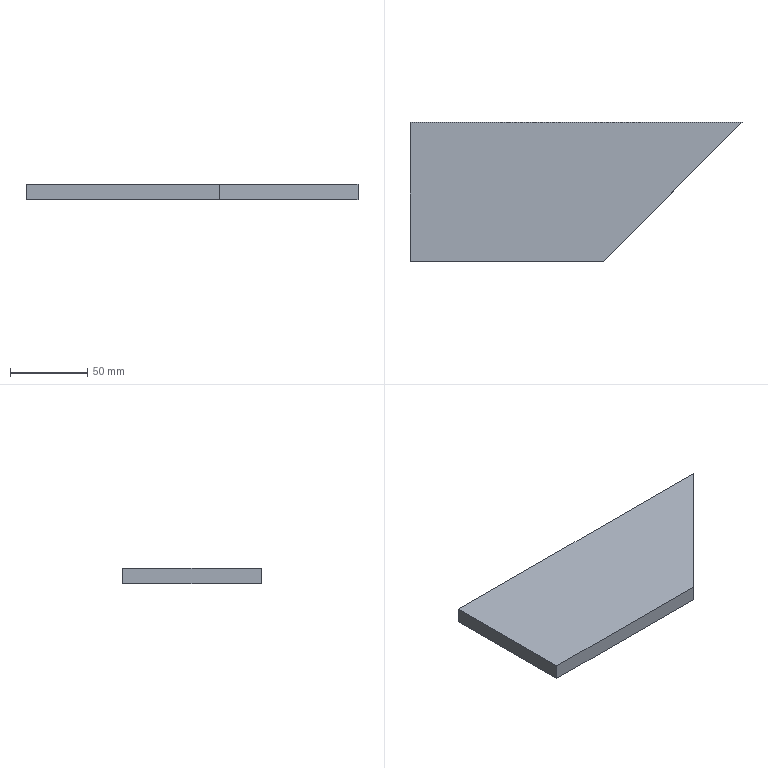Part | STEP file | 06-Reinforcing rib plate | 1 solid | 6 faces | box 215 x 90 x 10 mm | volume 153000 mm3 | plane 6
STEP:
#1=CARTESIAN_POINT('',(0.,0.,0.));
#2=DIRECTION('',(0.,0.,1.));
#3=DIRECTION('',(1.,0.,0.));
#4=AXIS2_PLACEMENT_3D('',#1,#2,#3);
#5=CARTESIAN_POINT('',(0.,0.,0.));
#6=VERTEX_POINT('',#5);
#7=CARTESIAN_POINT('',(0.,-90.,0.));
#8=VERTEX_POINT('',#7);
#9=CARTESIAN_POINT('',(0.,0.,0.));
#10=DIRECTION('',(0.,-1.,0.));
#11=VECTOR('',#10,1.);
#12=LINE('',#9,#11);
#13=CARTESIAN_POINT('',(0.,0.,10.));
#14=DIRECTION('',(1.,0.,0.));
#15=DIRECTION('',(0.,1.,0.));
#16=AXIS2_PLACEMENT_3D('',#13,#14,#15);
#17=PLANE('',#16);
#18=CARTESIAN_POINT('',(0.,-10.));
#19=DIRECTION('',(-1.,0.));
#20=VECTOR('',#19,1.);
#21=LINE('',#18,#20);
#22=(GEOMETRIC_REPRESENTATION_CONTEXT(2)PARAMETRIC_REPRESENTATION_CONTEXT()REPRESENTATION_CONTEXT('',''));
#23=DEFINITIONAL_REPRESENTATION('',(#21),#22);
#24=PCURVE('',#17,#23);
#25=CARTESIAN_POINT('',(0.,0.,0.));
#26=DIRECTION('',(0.,0.,1.));
#27=DIRECTION('',(1.,0.,0.));
#28=AXIS2_PLACEMENT_3D('',#25,#26,#27);
#29=PLANE('',#28);
#30=CARTESIAN_POINT('',(0.,0.));
#31=DIRECTION('',(0.,-1.));
#32=VECTOR('',#31,1.);
#33=LINE('',#30,#32);
#34=(GEOMETRIC_REPRESENTATION_CONTEXT(2)PARAMETRIC_REPRESENTATION_CONTEXT()REPRESENTATION_CONTEXT('',''));
#35=DEFINITIONAL_REPRESENTATION('',(#33),#34);
#36=PCURVE('',#29,#35);
#37=SURFACE_CURVE('',#12,(#24,#36),.PCURVE_S1.);
#38=EDGE_CURVE('',#6,#8,#37,.T.);
#39=ORIENTED_EDGE('',*,*,#38,.T.);
#40=CARTESIAN_POINT('',(0.,-90.,10.));
#41=VERTEX_POINT('',#40);
#42=CARTESIAN_POINT('',(0.,-90.,10.));
#43=DIRECTION('',(0.,0.,-1.));
#44=VECTOR('',#43,1.);
#45=LINE('',#42,#44);
#46=CARTESIAN_POINT('',(-90.,0.));
#47=DIRECTION('',(0.,-1.));
#48=VECTOR('',#47,1.);
#49=LINE('',#46,#48);
#50=(GEOMETRIC_REPRESENTATION_CONTEXT(2)PARAMETRIC_REPRESENTATION_CONTEXT()REPRESENTATION_CONTEXT('',''));
#51=DEFINITIONAL_REPRESENTATION('',(#49),#50);
#52=PCURVE('',#17,#51);
#53=CARTESIAN_POINT('',(0.,-90.,10.));
#54=DIRECTION('',(0.,1.,0.));
#55=DIRECTION('',(0.,0.,1.));
#56=AXIS2_PLACEMENT_3D('',#53,#54,#55);
#57=PLANE('',#56);
#58=CARTESIAN_POINT('',(0.,0.));
#59=DIRECTION('',(-1.,0.));
#60=VECTOR('',#59,1.);
#61=LINE('',#58,#60);
#62=(GEOMETRIC_REPRESENTATION_CONTEXT(2)PARAMETRIC_REPRESENTATION_CONTEXT()REPRESENTATION_CONTEXT('',''));
#63=DEFINITIONAL_REPRESENTATION('',(#61),#62);
#64=PCURVE('',#57,#63);
#65=SURFACE_CURVE('',#45,(#52,#64),.PCURVE_S1.);
#66=EDGE_CURVE('',#41,#8,#65,.T.);
#67=ORIENTED_EDGE('',*,*,#66,.F.);
#68=CARTESIAN_POINT('',(0.,0.,10.));
#69=VERTEX_POINT('',#68);
#70=CARTESIAN_POINT('',(0.,0.,10.));
#71=DIRECTION('',(0.,-1.,0.));
#72=VECTOR('',#71,1.);
#73=LINE('',#70,#72);
#74=CARTESIAN_POINT('',(0.,0.));
#75=DIRECTION('',(-1.,0.));
#76=VECTOR('',#75,1.);
#77=LINE('',#74,#76);
#78=(GEOMETRIC_REPRESENTATION_CONTEXT(2)PARAMETRIC_REPRESENTATION_CONTEXT()REPRESENTATION_CONTEXT('',''));
#79=DEFINITIONAL_REPRESENTATION('',(#77),#78);
#80=PCURVE('',#17,#79);
#81=CARTESIAN_POINT('',(0.,0.,10.));
#82=DIRECTION('',(0.,0.,1.));
#83=DIRECTION('',(1.,0.,0.));
#84=AXIS2_PLACEMENT_3D('',#81,#82,#83);
#85=PLANE('',#84);
#86=CARTESIAN_POINT('',(0.,0.));
#87=DIRECTION('',(0.,-1.));
#88=VECTOR('',#87,1.);
#89=LINE('',#86,#88);
#90=(GEOMETRIC_REPRESENTATION_CONTEXT(2)PARAMETRIC_REPRESENTATION_CONTEXT()REPRESENTATION_CONTEXT('',''));
#91=DEFINITIONAL_REPRESENTATION('',(#89),#90);
#92=PCURVE('',#85,#91);
#93=SURFACE_CURVE('',#73,(#80,#92),.PCURVE_S1.);
#94=EDGE_CURVE('',#69,#41,#93,.T.);
#95=ORIENTED_EDGE('',*,*,#94,.F.);
#96=CARTESIAN_POINT('',(0.,0.,10.));
#97=DIRECTION('',(0.,0.,-1.));
#98=VECTOR('',#97,1.);
#99=LINE('',#96,#98);
#100=CARTESIAN_POINT('',(0.,0.));
#101=DIRECTION('',(0.,-1.));
#102=VECTOR('',#101,1.);
#103=LINE('',#100,#102);
#104=(GEOMETRIC_REPRESENTATION_CONTEXT(2)PARAMETRIC_REPRESENTATION_CONTEXT()REPRESENTATION_CONTEXT('',''));
#105=DEFINITIONAL_REPRESENTATION('',(#103),#104);
#106=PCURVE('',#17,#105);
#107=CARTESIAN_POINT('',(0.,0.,10.));
#108=DIRECTION('',(0.,-1.,0.));
#109=DIRECTION('',(0.,0.,-1.));
#110=AXIS2_PLACEMENT_3D('',#107,#108,#109);
#111=PLANE('',#110);
#112=CARTESIAN_POINT('',(0.,0.));
#113=DIRECTION('',(1.,0.));
#114=VECTOR('',#113,1.);
#115=LINE('',#112,#114);
#116=(GEOMETRIC_REPRESENTATION_CONTEXT(2)PARAMETRIC_REPRESENTATION_CONTEXT()REPRESENTATION_CONTEXT('',''));
#117=DEFINITIONAL_REPRESENTATION('',(#115),#116);
#118=PCURVE('',#111,#117);
#119=SURFACE_CURVE('',#99,(#106,#118),.PCURVE_S1.);
#120=EDGE_CURVE('',#69,#6,#119,.T.);
#121=ORIENTED_EDGE('',*,*,#120,.T.);
#122=EDGE_LOOP('',(#39,#67,#95,#121));
#123=FACE_BOUND('',#122,.T.);
#124=ADVANCED_FACE('',(#123),#17,.F.);
#125=CARTESIAN_POINT('',(125.,-90.,0.));
#126=VERTEX_POINT('',#125);
#127=CARTESIAN_POINT('',(0.,-90.,0.));
#128=DIRECTION('',(1.,0.,0.));
#129=VECTOR('',#128,1.);
#130=LINE('',#127,#129);
#131=CARTESIAN_POINT('',(-10.,0.));
#132=DIRECTION('',(0.,1.));
#133=VECTOR('',#132,1.);
#134=LINE('',#131,#133);
#135=(GEOMETRIC_REPRESENTATION_CONTEXT(2)PARAMETRIC_REPRESENTATION_CONTEXT()REPRESENTATION_CONTEXT('',''));
#136=DEFINITIONAL_REPRESENTATION('',(#134),#135);
#137=PCURVE('',#57,#136);
#138=CARTESIAN_POINT('',(0.,-90.));
#139=DIRECTION('',(1.,0.));
#140=VECTOR('',#139,1.);
#141=LINE('',#138,#140);
#142=(GEOMETRIC_REPRESENTATION_CONTEXT(2)PARAMETRIC_REPRESENTATION_CONTEXT()REPRESENTATION_CONTEXT('',''));
#143=DEFINITIONAL_REPRESENTATION('',(#141),#142);
#144=PCURVE('',#29,#143);
#145=SURFACE_CURVE('',#130,(#137,#144),.PCURVE_S1.);
#146=EDGE_CURVE('',#8,#126,#145,.T.);
#147=ORIENTED_EDGE('',*,*,#146,.T.);
#148=CARTESIAN_POINT('',(125.,-90.,10.));
#149=VERTEX_POINT('',#148);
#150=CARTESIAN_POINT('',(125.,-90.,10.));
#151=DIRECTION('',(0.,0.,-1.));
#152=VECTOR('',#151,1.);
#153=LINE('',#150,#152);
#154=CARTESIAN_POINT('',(0.,125.));
#155=DIRECTION('',(-1.,0.));
#156=VECTOR('',#155,1.);
#157=LINE('',#154,#156);
#158=(GEOMETRIC_REPRESENTATION_CONTEXT(2)PARAMETRIC_REPRESENTATION_CONTEXT()REPRESENTATION_CONTEXT('',''));
#159=DEFINITIONAL_REPRESENTATION('',(#157),#158);
#160=PCURVE('',#57,#159);
#161=CARTESIAN_POINT('',(215.,0.,10.));
#162=DIRECTION('',(-0.7071,0.7071,0.));
#163=DIRECTION('',(-0.7071,-0.7071,0.));
#164=AXIS2_PLACEMENT_3D('',#161,#162,#163);
#165=PLANE('',#164);
#166=CARTESIAN_POINT('',(127.279,0.));
#167=DIRECTION('',(0.,-1.));
#168=VECTOR('',#167,1.);
#169=LINE('',#166,#168);
#170=(GEOMETRIC_REPRESENTATION_CONTEXT(2)PARAMETRIC_REPRESENTATION_CONTEXT()REPRESENTATION_CONTEXT('',''));
#171=DEFINITIONAL_REPRESENTATION('',(#169),#170);
#172=PCURVE('',#165,#171);
#173=SURFACE_CURVE('',#153,(#160,#172),.PCURVE_S1.);
#174=EDGE_CURVE('',#149,#126,#173,.T.);
#175=ORIENTED_EDGE('',*,*,#174,.F.);
#176=CARTESIAN_POINT('',(0.,-90.,10.));
#177=DIRECTION('',(1.,0.,0.));
#178=VECTOR('',#177,1.);
#179=LINE('',#176,#178);
#180=CARTESIAN_POINT('',(0.,0.));
#181=DIRECTION('',(0.,1.));
#182=VECTOR('',#181,1.);
#183=LINE('',#180,#182);
#184=(GEOMETRIC_REPRESENTATION_CONTEXT(2)PARAMETRIC_REPRESENTATION_CONTEXT()REPRESENTATION_CONTEXT('',''));
#185=DEFINITIONAL_REPRESENTATION('',(#183),#184);
#186=PCURVE('',#57,#185);
#187=CARTESIAN_POINT('',(0.,-90.));
#188=DIRECTION('',(1.,0.));
#189=VECTOR('',#188,1.);
#190=LINE('',#187,#189);
#191=(GEOMETRIC_REPRESENTATION_CONTEXT(2)PARAMETRIC_REPRESENTATION_CONTEXT()REPRESENTATION_CONTEXT('',''));
#192=DEFINITIONAL_REPRESENTATION('',(#190),#191);
#193=PCURVE('',#85,#192);
#194=SURFACE_CURVE('',#179,(#186,#193),.PCURVE_S1.);
#195=EDGE_CURVE('',#41,#149,#194,.T.);
#196=ORIENTED_EDGE('',*,*,#195,.F.);
#197=ORIENTED_EDGE('',*,*,#66,.T.);
#198=EDGE_LOOP('',(#147,#175,#196,#197));
#199=FACE_BOUND('',#198,.T.);
#200=ADVANCED_FACE('',(#199),#57,.F.);
#201=CARTESIAN_POINT('',(215.,0.,0.));
#202=VERTEX_POINT('',#201);
#203=CARTESIAN_POINT('',(215.,0.,0.));
#204=DIRECTION('',(0.7071,0.7071,0.));
#205=VECTOR('',#204,1.);
#206=LINE('',#203,#205);
#207=CARTESIAN_POINT('',(0.,-10.));
#208=DIRECTION('',(-1.,0.));
#209=VECTOR('',#208,1.);
#210=LINE('',#207,#209);
#211=(GEOMETRIC_REPRESENTATION_CONTEXT(2)PARAMETRIC_REPRESENTATION_CONTEXT()REPRESENTATION_CONTEXT('',''));
#212=DEFINITIONAL_REPRESENTATION('',(#210),#211);
#213=PCURVE('',#165,#212);
#214=CARTESIAN_POINT('',(215.,0.));
#215=DIRECTION('',(0.7071,0.7071));
#216=VECTOR('',#215,1.);
#217=LINE('',#214,#216);
#218=(GEOMETRIC_REPRESENTATION_CONTEXT(2)PARAMETRIC_REPRESENTATION_CONTEXT()REPRESENTATION_CONTEXT('',''));
#219=DEFINITIONAL_REPRESENTATION('',(#217),#218);
#220=PCURVE('',#29,#219);
#221=SURFACE_CURVE('',#206,(#213,#220),.PCURVE_S1.);
#222=EDGE_CURVE('',#126,#202,#221,.T.);
#223=ORIENTED_EDGE('',*,*,#222,.T.);
#224=CARTESIAN_POINT('',(215.,0.,10.));
#225=VERTEX_POINT('',#224);
#226=CARTESIAN_POINT('',(215.,0.,10.));
#227=DIRECTION('',(0.,0.,-1.));
#228=VECTOR('',#227,1.);
#229=LINE('',#226,#228);
#230=CARTESIAN_POINT('',(0.,0.));
#231=DIRECTION('',(0.,-1.));
#232=VECTOR('',#231,1.);
#233=LINE('',#230,#232);
#234=(GEOMETRIC_REPRESENTATION_CONTEXT(2)PARAMETRIC_REPRESENTATION_CONTEXT()REPRESENTATION_CONTEXT('',''));
#235=DEFINITIONAL_REPRESENTATION('',(#233),#234);
#236=PCURVE('',#165,#235);
#237=CARTESIAN_POINT('',(0.,215.));
#238=DIRECTION('',(1.,0.));
#239=VECTOR('',#238,1.);
#240=LINE('',#237,#239);
#241=(GEOMETRIC_REPRESENTATION_CONTEXT(2)PARAMETRIC_REPRESENTATION_CONTEXT()REPRESENTATION_CONTEXT('',''));
#242=DEFINITIONAL_REPRESENTATION('',(#240),#241);
#243=PCURVE('',#111,#242);
#244=SURFACE_CURVE('',#229,(#236,#243),.PCURVE_S1.);
#245=EDGE_CURVE('',#225,#202,#244,.T.);
#246=ORIENTED_EDGE('',*,*,#245,.F.);
#247=CARTESIAN_POINT('',(215.,0.,10.));
#248=DIRECTION('',(0.7071,0.7071,0.));
#249=VECTOR('',#248,1.);
#250=LINE('',#247,#249);
#251=CARTESIAN_POINT('',(0.,0.));
#252=DIRECTION('',(-1.,0.));
#253=VECTOR('',#252,1.);
#254=LINE('',#251,#253);
#255=(GEOMETRIC_REPRESENTATION_CONTEXT(2)PARAMETRIC_REPRESENTATION_CONTEXT()REPRESENTATION_CONTEXT('',''));
#256=DEFINITIONAL_REPRESENTATION('',(#254),#255);
#257=PCURVE('',#165,#256);
#258=CARTESIAN_POINT('',(215.,0.));
#259=DIRECTION('',(0.7071,0.7071));
#260=VECTOR('',#259,1.);
#261=LINE('',#258,#260);
#262=(GEOMETRIC_REPRESENTATION_CONTEXT(2)PARAMETRIC_REPRESENTATION_CONTEXT()REPRESENTATION_CONTEXT('',''));
#263=DEFINITIONAL_REPRESENTATION('',(#261),#262);
#264=PCURVE('',#85,#263);
#265=SURFACE_CURVE('',#250,(#257,#264),.PCURVE_S1.);
#266=EDGE_CURVE('',#149,#225,#265,.T.);
#267=ORIENTED_EDGE('',*,*,#266,.F.);
#268=ORIENTED_EDGE('',*,*,#174,.T.);
#269=EDGE_LOOP('',(#223,#246,#267,#268));
#270=FACE_BOUND('',#269,.T.);
#271=ADVANCED_FACE('',(#270),#165,.F.);
#272=CARTESIAN_POINT('',(0.,0.,0.));
#273=DIRECTION('',(-1.,0.,0.));
#274=VECTOR('',#273,1.);
#275=LINE('',#272,#274);
#276=CARTESIAN_POINT('',(10.,0.));
#277=DIRECTION('',(0.,-1.));
#278=VECTOR('',#277,1.);
#279=LINE('',#276,#278);
#280=(GEOMETRIC_REPRESENTATION_CONTEXT(2)PARAMETRIC_REPRESENTATION_CONTEXT()REPRESENTATION_CONTEXT('',''));
#281=DEFINITIONAL_REPRESENTATION('',(#279),#280);
#282=PCURVE('',#111,#281);
#283=CARTESIAN_POINT('',(0.,0.));
#284=DIRECTION('',(-1.,0.));
#285=VECTOR('',#284,1.);
#286=LINE('',#283,#285);
#287=(GEOMETRIC_REPRESENTATION_CONTEXT(2)PARAMETRIC_REPRESENTATION_CONTEXT()REPRESENTATION_CONTEXT('',''));
#288=DEFINITIONAL_REPRESENTATION('',(#286),#287);
#289=PCURVE('',#29,#288);
#290=SURFACE_CURVE('',#275,(#282,#289),.PCURVE_S1.);
#291=EDGE_CURVE('',#202,#6,#290,.T.);
#292=ORIENTED_EDGE('',*,*,#291,.T.);
#293=ORIENTED_EDGE('',*,*,#120,.F.);
#294=CARTESIAN_POINT('',(0.,0.,10.));
#295=DIRECTION('',(-1.,0.,0.));
#296=VECTOR('',#295,1.);
#297=LINE('',#294,#296);
#298=CARTESIAN_POINT('',(0.,0.));
#299=DIRECTION('',(0.,-1.));
#300=VECTOR('',#299,1.);
#301=LINE('',#298,#300);
#302=(GEOMETRIC_REPRESENTATION_CONTEXT(2)PARAMETRIC_REPRESENTATION_CONTEXT()REPRESENTATION_CONTEXT('',''));
#303=DEFINITIONAL_REPRESENTATION('',(#301),#302);
#304=PCURVE('',#111,#303);
#305=CARTESIAN_POINT('',(0.,0.));
#306=DIRECTION('',(-1.,0.));
#307=VECTOR('',#306,1.);
#308=LINE('',#305,#307);
#309=(GEOMETRIC_REPRESENTATION_CONTEXT(2)PARAMETRIC_REPRESENTATION_CONTEXT()REPRESENTATION_CONTEXT('',''));
#310=DEFINITIONAL_REPRESENTATION('',(#308),#309);
#311=PCURVE('',#85,#310);
#312=SURFACE_CURVE('',#297,(#304,#311),.PCURVE_S1.);
#313=EDGE_CURVE('',#225,#69,#312,.T.);
#314=ORIENTED_EDGE('',*,*,#313,.F.);
#315=ORIENTED_EDGE('',*,*,#245,.T.);
#316=EDGE_LOOP('',(#292,#293,#314,#315));
#317=FACE_BOUND('',#316,.T.);
#318=ADVANCED_FACE('',(#317),#111,.F.);
#319=ORIENTED_EDGE('',*,*,#94,.T.);
#320=ORIENTED_EDGE('',*,*,#195,.T.);
#321=ORIENTED_EDGE('',*,*,#266,.T.);
#322=ORIENTED_EDGE('',*,*,#313,.T.);
#323=EDGE_LOOP('',(#319,#320,#321,#322));
#324=FACE_BOUND('',#323,.T.);
#325=ADVANCED_FACE('',(#324),#85,.T.);
#326=ORIENTED_EDGE('',*,*,#38,.F.);
#327=ORIENTED_EDGE('',*,*,#291,.F.);
#328=ORIENTED_EDGE('',*,*,#222,.F.);
#329=ORIENTED_EDGE('',*,*,#146,.F.);
#330=EDGE_LOOP('',(#326,#327,#328,#329));
#331=FACE_BOUND('',#330,.T.);
#332=ADVANCED_FACE('',(#331),#29,.F.);
#333=CLOSED_SHELL('',(#124,#200,#271,#318,#325,#332));
#334=MANIFOLD_SOLID_BREP('',#333);
#335=(LENGTH_UNIT()NAMED_UNIT(*)SI_UNIT(.MILLI.,.METRE.));
#336=UNCERTAINTY_MEASURE_WITH_UNIT(LENGTH_MEASURE(0.0000001),#335,'','');
#337=(NAMED_UNIT(*)PLANE_ANGLE_UNIT()SI_UNIT($,.RADIAN.));
#338=(NAMED_UNIT(*)SI_UNIT($,.STERADIAN.)SOLID_ANGLE_UNIT());
#339=(GEOMETRIC_REPRESENTATION_CONTEXT(3)GLOBAL_UNCERTAINTY_ASSIGNED_CONTEXT((#336))GLOBAL_UNIT_ASSIGNED_CONTEXT((#335,#337,#338))REPRESENTATION_CONTEXT('',''));
#340=ADVANCED_BREP_SHAPE_REPRESENTATION('',(#4,#334),#339);